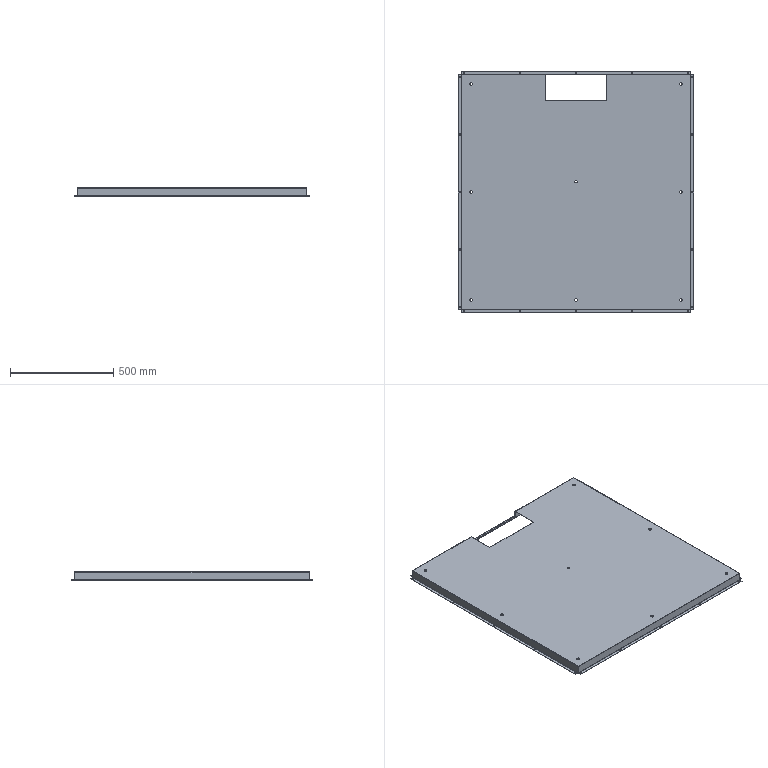Part | 1 solid | 186 faces | box 1139 x 1169 x 40 mm | volume 1452478 mm3 | plane 94 | cylinder 84 | spline 8 | commonest cylinder face diameters 7 x50 14 x14 0.4 x9 2.4 x9 11 x2